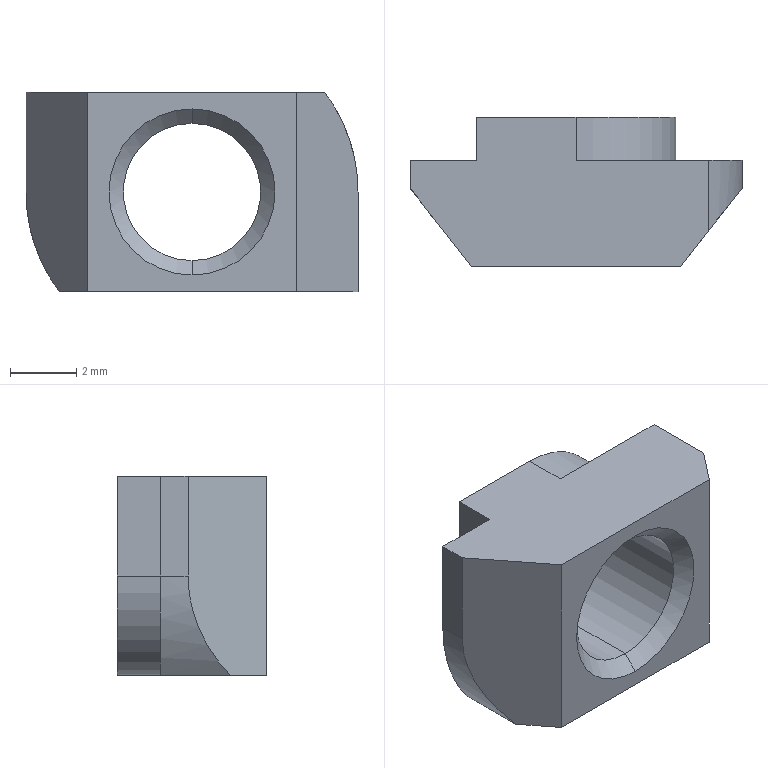Part | SolidWorks | features ICE 2, Extrusion 1, Fillet 1, RevCut 1 | 1 solid | 22 faces | box 10 x 4.5 x 6 mm | volume 142.178 mm3 | plane 12 | cylinder 6 | cone 4 | commonest cylinder face diameters 4.134 x2 6 x2 10 x2
STEP:
#1=CARTESIAN_POINT('',(0.,4.067,5.067));
#2=VERTEX_POINT('',#1);
#3=CARTESIAN_POINT('',(0.,4.067,0.933));
#4=VERTEX_POINT('',#3);
#5=CARTESIAN_POINT('',(0.,4.067,3.));
#6=DIRECTION('',(0.,-1.,0.));
#7=DIRECTION('',(0.,0.,-1.));
#8=AXIS2_PLACEMENT_3D('',#5,#6,#7);
#9=CIRCLE('',#8,2.067);
#10=EDGE_CURVE('',#2,#4,#9,.T.);
#11=ORIENTED_EDGE('',*,*,#10,.T.);
#12=CARTESIAN_POINT('',(0.,4.5,0.5));
#13=VERTEX_POINT('',#12);
#14=CARTESIAN_POINT('',(0.,4.5,0.5));
#15=DIRECTION('',(0.,0.7071,-0.7071));
#16=VECTOR('',#15,1000.);
#17=LINE('',#14,#16);
#18=EDGE_CURVE('',#4,#13,#17,.T.);
#19=ORIENTED_EDGE('',*,*,#18,.T.);
#20=CARTESIAN_POINT('',(0.,4.5,5.5));
#21=VERTEX_POINT('',#20);
#22=CARTESIAN_POINT('',(0.,4.5,3.));
#23=DIRECTION('',(0.,-1.,0.));
#24=DIRECTION('',(0.,0.,-1.));
#25=AXIS2_PLACEMENT_3D('',#22,#23,#24);
#26=CIRCLE('',#25,2.5);
#27=EDGE_CURVE('',#21,#13,#26,.T.);
#28=ORIENTED_EDGE('',*,*,#27,.F.);
#29=CARTESIAN_POINT('',(0.,4.5,5.5));
#30=DIRECTION('',(0.,0.7071,0.7071));
#31=VECTOR('',#30,1000.);
#32=LINE('',#29,#31);
#33=EDGE_CURVE('',#2,#21,#32,.T.);
#34=ORIENTED_EDGE('',*,*,#33,.F.);
#35=EDGE_LOOP('',(#11,#19,#28,#34));
#36=FACE_OUTER_BOUND('',#35,.T.);
#37=CARTESIAN_POINT('',(0.,4.5,3.));
#38=DIRECTION('',(0.,1.,0.));
#39=DIRECTION('',(0.,0.,1.));
#40=AXIS2_PLACEMENT_3D('',#37,#38,#39);
#41=CONICAL_SURFACE('',#40,2.5,0.7854);
#42=ADVANCED_FACE('',(#36),#41,.F.);
#43=ORIENTED_EDGE('',*,*,#10,.F.);
#44=CARTESIAN_POINT('',(0.,0.433,5.067));
#45=VERTEX_POINT('',#44);
#46=CARTESIAN_POINT('',(0.,50.,5.067));
#47=DIRECTION('',(0.,-1.,0.));
#48=VECTOR('',#47,1000.);
#49=LINE('',#46,#48);
#50=EDGE_CURVE('',#2,#45,#49,.T.);
#51=ORIENTED_EDGE('',*,*,#50,.T.);
#52=CARTESIAN_POINT('',(0.,0.433,0.933));
#53=VERTEX_POINT('',#52);
#54=CARTESIAN_POINT('',(0.,0.433,3.));
#55=DIRECTION('',(0.,-1.,0.));
#56=DIRECTION('',(0.,0.,-1.));
#57=AXIS2_PLACEMENT_3D('',#54,#55,#56);
#58=CIRCLE('',#57,2.067);
#59=EDGE_CURVE('',#45,#53,#58,.T.);
#60=ORIENTED_EDGE('',*,*,#59,.T.);
#61=CARTESIAN_POINT('',(0.,50.,0.933));
#62=DIRECTION('',(0.,-1.,0.));
#63=VECTOR('',#62,1000.);
#64=LINE('',#61,#63);
#65=EDGE_CURVE('',#4,#53,#64,.T.);
#66=ORIENTED_EDGE('',*,*,#65,.F.);
#67=EDGE_LOOP('',(#43,#51,#60,#66));
#68=FACE_OUTER_BOUND('',#67,.T.);
#69=CARTESIAN_POINT('',(0.,50.,3.));
#70=DIRECTION('',(0.,-1.,0.));
#71=DIRECTION('',(0.,0.,-1.));
#72=AXIS2_PLACEMENT_3D('',#69,#70,#71);
#73=CYLINDRICAL_SURFACE('',#72,2.067);
#74=ADVANCED_FACE('',(#68),#73,.F.);
#75=ORIENTED_EDGE('',*,*,#59,.F.);
#76=CARTESIAN_POINT('',(0.,0.,5.5));
#77=VERTEX_POINT('',#76);
#78=CARTESIAN_POINT('',(0.,0.433,5.067));
#79=DIRECTION('',(0.,-0.7071,0.7071));
#80=VECTOR('',#79,1000.);
#81=LINE('',#78,#80);
#82=EDGE_CURVE('',#45,#77,#81,.T.);
#83=ORIENTED_EDGE('',*,*,#82,.T.);
#84=CARTESIAN_POINT('',(0.,0.,0.5));
#85=VERTEX_POINT('',#84);
#86=CARTESIAN_POINT('',(0.,0.,3.));
#87=DIRECTION('',(0.,-1.,0.));
#88=DIRECTION('',(0.,0.,-1.));
#89=AXIS2_PLACEMENT_3D('',#86,#87,#88);
#90=CIRCLE('',#89,2.5);
#91=EDGE_CURVE('',#77,#85,#90,.T.);
#92=ORIENTED_EDGE('',*,*,#91,.T.);
#93=CARTESIAN_POINT('',(0.,0.433,0.933));
#94=DIRECTION('',(0.,-0.7071,-0.7071));
#95=VECTOR('',#94,1000.);
#96=LINE('',#93,#95);
#97=EDGE_CURVE('',#53,#85,#96,.T.);
#98=ORIENTED_EDGE('',*,*,#97,.F.);
#99=EDGE_LOOP('',(#75,#83,#92,#98));
#100=FACE_OUTER_BOUND('',#99,.T.);
#101=CARTESIAN_POINT('',(0.,0.433,3.));
#102=DIRECTION('',(0.,-1.,0.));
#103=DIRECTION('',(0.,0.,-1.));
#104=AXIS2_PLACEMENT_3D('',#101,#102,#103);
#105=CONICAL_SURFACE('',#104,2.067,0.7854);
#106=ADVANCED_FACE('',(#100),#105,.F.);
#107=CARTESIAN_POINT('',(-5.,3.2,6.));
#108=VERTEX_POINT('',#107);
#109=CARTESIAN_POINT('',(-5.,3.2,3.));
#110=VERTEX_POINT('',#109);
#111=CARTESIAN_POINT('',(-5.,3.2,6.));
#112=DIRECTION('',(0.,0.,-1.));
#113=VECTOR('',#112,1000.);
#114=LINE('',#111,#113);
#115=EDGE_CURVE('',#108,#110,#114,.T.);
#116=ORIENTED_EDGE('',*,*,#115,.T.);
#117=CARTESIAN_POINT('',(-5.,2.368,3.));
#118=VERTEX_POINT('',#117);
#119=CARTESIAN_POINT('',(-5.,0.,3.));
#120=DIRECTION('',(0.,1.,0.));
#121=VECTOR('',#120,1000.);
#122=LINE('',#119,#121);
#123=EDGE_CURVE('',#118,#110,#122,.T.);
#124=ORIENTED_EDGE('',*,*,#123,.F.);
#125=CARTESIAN_POINT('',(-5.,2.368,6.));
#126=VERTEX_POINT('',#125);
#127=CARTESIAN_POINT('',(-5.,2.368,6.));
#128=DIRECTION('',(0.,0.,-1.));
#129=VECTOR('',#128,1000.);
#130=LINE('',#127,#129);
#131=EDGE_CURVE('',#126,#118,#130,.T.);
#132=ORIENTED_EDGE('',*,*,#131,.F.);
#133=CARTESIAN_POINT('',(-5.,3.2,6.));
#134=DIRECTION('',(0.,-1.,0.));
#135=VECTOR('',#134,1000.);
#136=LINE('',#133,#135);
#137=EDGE_CURVE('',#108,#126,#136,.T.);
#138=ORIENTED_EDGE('',*,*,#137,.F.);
#139=EDGE_LOOP('',(#116,#124,#132,#138));
#140=FACE_OUTER_BOUND('',#139,.T.);
#141=CARTESIAN_POINT('',(-5.,3.2,6.));
#142=DIRECTION('',(1.,0.,0.));
#143=DIRECTION('',(0.,0.,-1.));
#144=AXIS2_PLACEMENT_3D('',#141,#142,#143);
#145=PLANE('',#144);
#146=ADVANCED_FACE('',(#140),#145,.F.);
#147=ORIENTED_EDGE('',*,*,#131,.T.);
#148=CARTESIAN_POINT('',(-4.,1.088,0.));
#149=VERTEX_POINT('',#148);
#150=CARTESIAN_POINT('',(-5.,2.368,3.));
#151=CARTESIAN_POINT('',(-5.,2.368,1.909));
#152=CARTESIAN_POINT('',(-4.655,1.926,0.8731));
#153=CARTESIAN_POINT('',(-4.,1.088,0.));
#154=(BOUNDED_CURVE()B_SPLINE_CURVE(3,(#150,#151,#152,#153),.UNSPECIFIED.,.F.,.F.)B_SPLINE_CURVE_WITH_KNOTS((4,4),(0.,0.6435),.UNSPECIFIED.)CURVE()GEOMETRIC_REPRESENTATION_ITEM()RATIONAL_B_SPLINE_CURVE((1.,0.9658,0.9658,1.))REPRESENTATION_ITEM(''));
#155=EDGE_CURVE('',#118,#149,#154,.T.);
#156=ORIENTED_EDGE('',*,*,#155,.T.);
#157=CARTESIAN_POINT('',(-3.15,0.,0.));
#158=VERTEX_POINT('',#157);
#159=CARTESIAN_POINT('',(-5.,2.368,0.));
#160=DIRECTION('',(0.6157,-0.788,0.));
#161=VECTOR('',#160,1000.);
#162=LINE('',#159,#161);
#163=EDGE_CURVE('',#149,#158,#162,.T.);
#164=ORIENTED_EDGE('',*,*,#163,.T.);
#165=CARTESIAN_POINT('',(-3.15,0.,6.));
#166=VERTEX_POINT('',#165);
#167=CARTESIAN_POINT('',(-3.15,0.,6.));
#168=DIRECTION('',(0.,0.,-1.));
#169=VECTOR('',#168,1000.);
#170=LINE('',#167,#169);
#171=EDGE_CURVE('',#166,#158,#170,.T.);
#172=ORIENTED_EDGE('',*,*,#171,.F.);
#173=CARTESIAN_POINT('',(-5.,2.368,6.));
#174=DIRECTION('',(0.6157,-0.788,0.));
#175=VECTOR('',#174,1000.);
#176=LINE('',#173,#175);
#177=EDGE_CURVE('',#126,#166,#176,.T.);
#178=ORIENTED_EDGE('',*,*,#177,.F.);
#179=EDGE_LOOP('',(#147,#156,#164,#172,#178));
#180=FACE_OUTER_BOUND('',#179,.T.);
#181=CARTESIAN_POINT('',(-5.,2.368,6.));
#182=DIRECTION('',(0.788,0.6157,0.));
#183=DIRECTION('',(-0.6157,0.788,0.));
#184=AXIS2_PLACEMENT_3D('',#181,#182,#183);
#185=PLANE('',#184);
#186=ADVANCED_FACE('',(#180),#185,.F.);
#187=CARTESIAN_POINT('',(0.,0.,3.));
#188=DIRECTION('',(0.,-1.,0.));
#189=DIRECTION('',(0.,0.,-1.));
#190=AXIS2_PLACEMENT_3D('',#187,#188,#189);
#191=CIRCLE('',#190,2.5);
#192=EDGE_CURVE('',#85,#77,#191,.T.);
#193=ORIENTED_EDGE('',*,*,#192,.F.);
#194=ORIENTED_EDGE('',*,*,#91,.F.);
#195=EDGE_LOOP('',(#193,#194));
#196=FACE_BOUND('',#195,.T.);
#197=CARTESIAN_POINT('',(3.15,0.,0.));
#198=VERTEX_POINT('',#197);
#199=CARTESIAN_POINT('',(-3.15,0.,0.));
#200=DIRECTION('',(1.,0.,0.));
#201=VECTOR('',#200,1000.);
#202=LINE('',#199,#201);
#203=EDGE_CURVE('',#158,#198,#202,.T.);
#204=ORIENTED_EDGE('',*,*,#203,.T.);
#205=CARTESIAN_POINT('',(3.15,0.,6.));
#206=VERTEX_POINT('',#205);
#207=CARTESIAN_POINT('',(3.15,0.,6.));
#208=DIRECTION('',(0.,0.,-1.));
#209=VECTOR('',#208,1000.);
#210=LINE('',#207,#209);
#211=EDGE_CURVE('',#206,#198,#210,.T.);
#212=ORIENTED_EDGE('',*,*,#211,.F.);
#213=CARTESIAN_POINT('',(-3.15,0.,6.));
#214=DIRECTION('',(1.,0.,0.));
#215=VECTOR('',#214,1000.);
#216=LINE('',#213,#215);
#217=EDGE_CURVE('',#166,#206,#216,.T.);
#218=ORIENTED_EDGE('',*,*,#217,.F.);
#219=ORIENTED_EDGE('',*,*,#171,.T.);
#220=EDGE_LOOP('',(#204,#212,#218,#219));
#221=FACE_OUTER_BOUND('',#220,.T.);
#222=CARTESIAN_POINT('',(-3.15,0.,6.));
#223=DIRECTION('',(0.,1.,0.));
#224=DIRECTION('',(0.,0.,1.));
#225=AXIS2_PLACEMENT_3D('',#222,#223,#224);
#226=PLANE('',#225);
#227=ADVANCED_FACE('',(#196,#221),#226,.F.);
#228=CARTESIAN_POINT('',(5.,2.368,3.));
#229=VERTEX_POINT('',#228);
#230=CARTESIAN_POINT('',(5.,2.368,0.));
#231=VERTEX_POINT('',#230);
#232=CARTESIAN_POINT('',(5.,2.368,6.));
#233=DIRECTION('',(0.,0.,-1.));
#234=VECTOR('',#233,1000.);
#235=LINE('',#232,#234);
#236=EDGE_CURVE('',#229,#231,#235,.T.);
#237=ORIENTED_EDGE('',*,*,#236,.F.);
#238=CARTESIAN_POINT('',(4.,1.088,6.));
#239=VERTEX_POINT('',#238);
#240=CARTESIAN_POINT('',(5.,2.368,3.));
#241=CARTESIAN_POINT('',(5.,2.368,4.091));
#242=CARTESIAN_POINT('',(4.655,1.926,5.127));
#243=CARTESIAN_POINT('',(4.,1.088,6.));
#244=(BOUNDED_CURVE()B_SPLINE_CURVE(3,(#240,#241,#242,#243),.UNSPECIFIED.,.F.,.F.)B_SPLINE_CURVE_WITH_KNOTS((4,4),(0.,0.6435),.UNSPECIFIED.)CURVE()GEOMETRIC_REPRESENTATION_ITEM()RATIONAL_B_SPLINE_CURVE((1.,0.9658,0.9658,1.))REPRESENTATION_ITEM(''));
#245=EDGE_CURVE('',#229,#239,#244,.T.);
#246=ORIENTED_EDGE('',*,*,#245,.T.);
#247=CARTESIAN_POINT('',(3.15,0.,6.));
#248=DIRECTION('',(0.6157,0.788,0.));
#249=VECTOR('',#248,1000.);
#250=LINE('',#247,#249);
#251=EDGE_CURVE('',#206,#239,#250,.T.);
#252=ORIENTED_EDGE('',*,*,#251,.F.);
#253=ORIENTED_EDGE('',*,*,#211,.T.);
#254=CARTESIAN_POINT('',(3.15,0.,0.));
#255=DIRECTION('',(0.6157,0.788,0.));
#256=VECTOR('',#255,1000.);
#257=LINE('',#254,#256);
#258=EDGE_CURVE('',#198,#231,#257,.T.);
#259=ORIENTED_EDGE('',*,*,#258,.T.);
#260=EDGE_LOOP('',(#237,#246,#252,#253,#259));
#261=FACE_OUTER_BOUND('',#260,.T.);
#262=CARTESIAN_POINT('',(3.15,0.,6.));
#263=DIRECTION('',(-0.788,0.6157,0.));
#264=DIRECTION('',(-0.6157,-0.788,0.));
#265=AXIS2_PLACEMENT_3D('',#262,#263,#264);
#266=PLANE('',#265);
#267=ADVANCED_FACE('',(#261),#266,.F.);
#268=CARTESIAN_POINT('',(5.,3.2,3.));
#269=VERTEX_POINT('',#268);
#270=CARTESIAN_POINT('',(5.,3.2,0.));
#271=VERTEX_POINT('',#270);
#272=CARTESIAN_POINT('',(5.,3.2,6.));
#273=DIRECTION('',(0.,0.,-1.));
#274=VECTOR('',#273,1000.);
#275=LINE('',#272,#274);
#276=EDGE_CURVE('',#269,#271,#275,.T.);
#277=ORIENTED_EDGE('',*,*,#276,.F.);
#278=CARTESIAN_POINT('',(5.,0.,3.));
#279=DIRECTION('',(0.,1.,0.));
#280=VECTOR('',#279,1000.);
#281=LINE('',#278,#280);
#282=EDGE_CURVE('',#229,#269,#281,.T.);
#283=ORIENTED_EDGE('',*,*,#282,.F.);
#284=ORIENTED_EDGE('',*,*,#236,.T.);
#285=CARTESIAN_POINT('',(5.,2.368,0.));
#286=DIRECTION('',(0.,1.,0.));
#287=VECTOR('',#286,1000.);
#288=LINE('',#285,#287);
#289=EDGE_CURVE('',#231,#271,#288,.T.);
#290=ORIENTED_EDGE('',*,*,#289,.T.);
#291=EDGE_LOOP('',(#277,#283,#284,#290));
#292=FACE_OUTER_BOUND('',#291,.T.);
#293=CARTESIAN_POINT('',(5.,2.368,6.));
#294=DIRECTION('',(-1.,0.,0.));
#295=DIRECTION('',(0.,0.,1.));
#296=AXIS2_PLACEMENT_3D('',#293,#294,#295);
#297=PLANE('',#296);
#298=ADVANCED_FACE('',(#292),#297,.F.);
#299=CARTESIAN_POINT('',(4.,3.2,6.));
#300=VERTEX_POINT('',#299);
#301=CARTESIAN_POINT('',(0.,3.2,6.));
#302=VERTEX_POINT('',#301);
#303=CARTESIAN_POINT('',(5.,3.2,6.));
#304=DIRECTION('',(-1.,0.,0.));
#305=VECTOR('',#304,1000.);
#306=LINE('',#303,#305);
#307=EDGE_CURVE('',#300,#302,#306,.T.);
#308=ORIENTED_EDGE('',*,*,#307,.F.);
#309=CARTESIAN_POINT('',(0.,3.2,3.));
#310=DIRECTION('',(0.,1.,0.));
#311=DIRECTION('',(0.,0.,-1.));
#312=AXIS2_PLACEMENT_3D('',#309,#310,#311);
#313=CIRCLE('',#312,5.);
#314=EDGE_CURVE('',#300,#269,#313,.T.);
#315=ORIENTED_EDGE('',*,*,#314,.T.);
#316=ORIENTED_EDGE('',*,*,#276,.T.);
#317=CARTESIAN_POINT('',(3.,3.2,0.));
#318=VERTEX_POINT('',#317);
#319=CARTESIAN_POINT('',(5.,3.2,0.));
#320=DIRECTION('',(-1.,0.,0.));
#321=VECTOR('',#320,1000.);
#322=LINE('',#319,#321);
#323=EDGE_CURVE('',#271,#318,#322,.T.);
#324=ORIENTED_EDGE('',*,*,#323,.T.);
#325=CARTESIAN_POINT('',(3.,3.2,3.));
#326=VERTEX_POINT('',#325);
#327=CARTESIAN_POINT('',(3.,3.2,6.));
#328=DIRECTION('',(0.,0.,-1.));
#329=VECTOR('',#328,1000.);
#330=LINE('',#327,#329);
#331=EDGE_CURVE('',#326,#318,#330,.T.);
#332=ORIENTED_EDGE('',*,*,#331,.F.);
#333=CARTESIAN_POINT('',(0.,3.2,3.));
#334=DIRECTION('',(0.,-1.,0.));
#335=DIRECTION('',(0.,0.,-1.));
#336=AXIS2_PLACEMENT_3D('',#333,#334,#335);
#337=CIRCLE('',#336,3.);
#338=EDGE_CURVE('',#326,#302,#337,.T.);
#339=ORIENTED_EDGE('',*,*,#338,.T.);
#340=EDGE_LOOP('',(#308,#315,#316,#324,#332,#339));
#341=FACE_OUTER_BOUND('',#340,.T.);
#342=CARTESIAN_POINT('',(5.,3.2,6.));
#343=DIRECTION('',(0.,-1.,0.));
#344=DIRECTION('',(0.,0.,-1.));
#345=AXIS2_PLACEMENT_3D('',#342,#343,#344);
#346=PLANE('',#345);
#347=ADVANCED_FACE('',(#341),#346,.F.);
#348=CARTESIAN_POINT('',(3.,4.5,3.));
#349=VERTEX_POINT('',#348);
#350=CARTESIAN_POINT('',(3.,4.5,0.));
#351=VERTEX_POINT('',#350);
#352=CARTESIAN_POINT('',(3.,4.5,6.));
#353=DIRECTION('',(0.,0.,-1.));
#354=VECTOR('',#353,1000.);
#355=LINE('',#352,#354);
#356=EDGE_CURVE('',#349,#351,#355,.T.);
#357=ORIENTED_EDGE('',*,*,#356,.F.);
#358=CARTESIAN_POINT('',(3.,3.2,3.));
#359=DIRECTION('',(0.,-1.,0.));
#360=VECTOR('',#359,1000.);
#361=LINE('',#358,#360);
#362=EDGE_CURVE('',#349,#326,#361,.T.);
#363=ORIENTED_EDGE('',*,*,#362,.T.);
#364=ORIENTED_EDGE('',*,*,#331,.T.);
#365=CARTESIAN_POINT('',(3.,3.2,0.));
#366=DIRECTION('',(0.,1.,0.));
#367=VECTOR('',#366,1000.);
#368=LINE('',#365,#367);
#369=EDGE_CURVE('',#318,#351,#368,.T.);
#370=ORIENTED_EDGE('',*,*,#369,.T.);
#371=EDGE_LOOP('',(#357,#363,#364,#370));
#372=FACE_OUTER_BOUND('',#371,.T.);
#373=CARTESIAN_POINT('',(3.,3.2,6.));
#374=DIRECTION('',(-1.,0.,0.));
#375=DIRECTION('',(0.,0.,1.));
#376=AXIS2_PLACEMENT_3D('',#373,#374,#375);
#377=PLANE('',#376);
#378=ADVANCED_FACE('',(#372),#377,.F.);
#379=ORIENTED_EDGE('',*,*,#27,.T.);
#380=CARTESIAN_POINT('',(0.,4.5,3.));
#381=DIRECTION('',(0.,-1.,0.));
#382=DIRECTION('',(0.,0.,-1.));
#383=AXIS2_PLACEMENT_3D('',#380,#381,#382);
#384=CIRCLE('',#383,2.5);
#385=EDGE_CURVE('',#13,#21,#384,.T.);
#386=ORIENTED_EDGE('',*,*,#385,.T.);
#387=EDGE_LOOP('',(#379,#386));
#388=FACE_BOUND('',#387,.T.);
#389=CARTESIAN_POINT('',(0.,4.5,6.));
#390=VERTEX_POINT('',#389);
#391=CARTESIAN_POINT('',(-3.,4.5,6.));
#392=VERTEX_POINT('',#391);
#393=CARTESIAN_POINT('',(3.,4.5,6.));
#394=DIRECTION('',(-1.,0.,0.));
#395=VECTOR('',#394,1000.);
#396=LINE('',#393,#395);
#397=EDGE_CURVE('',#390,#392,#396,.T.);
#398=ORIENTED_EDGE('',*,*,#397,.F.);
#399=CARTESIAN_POINT('',(0.,4.5,3.));
#400=DIRECTION('',(0.,1.,0.));
#401=DIRECTION('',(0.,0.,-1.));
#402=AXIS2_PLACEMENT_3D('',#399,#400,#401);
#403=CIRCLE('',#402,3.);
#404=EDGE_CURVE('',#390,#349,#403,.T.);
#405=ORIENTED_EDGE('',*,*,#404,.T.);
#406=ORIENTED_EDGE('',*,*,#356,.T.);
#407=CARTESIAN_POINT('',(0.,4.5,0.));
#408=VERTEX_POINT('',#407);
#409=CARTESIAN_POINT('',(3.,4.5,0.));
#410=DIRECTION('',(-1.,0.,0.));
#411=VECTOR('',#410,1000.);
#412=LINE('',#409,#411);
#413=EDGE_CURVE('',#351,#408,#412,.T.);
#414=ORIENTED_EDGE('',*,*,#413,.T.);
#415=CARTESIAN_POINT('',(-3.,4.5,3.));
#416=VERTEX_POINT('',#415);
#417=CARTESIAN_POINT('',(0.,4.5,3.));
#418=DIRECTION('',(0.,1.,0.));
#419=DIRECTION('',(0.,0.,-1.));
#420=AXIS2_PLACEMENT_3D('',#417,#418,#419);
#421=CIRCLE('',#420,3.);
#422=EDGE_CURVE('',#408,#416,#421,.T.);
#423=ORIENTED_EDGE('',*,*,#422,.T.);
#424=CARTESIAN_POINT('',(-3.,4.5,6.));
#425=DIRECTION('',(0.,0.,-1.));
#426=VECTOR('',#425,1000.);
#427=LINE('',#424,#426);
#428=EDGE_CURVE('',#392,#416,#427,.T.);
#429=ORIENTED_EDGE('',*,*,#428,.F.);
#430=EDGE_LOOP('',(#398,#405,#406,#414,#423,#429));
#431=FACE_OUTER_BOUND('',#430,.T.);
#432=CARTESIAN_POINT('',(3.,4.5,6.));
#433=DIRECTION('',(0.,-1.,0.));
#434=DIRECTION('',(0.,0.,-1.));
#435=AXIS2_PLACEMENT_3D('',#432,#433,#434);
#436=PLANE('',#435);
#437=ADVANCED_FACE('',(#388,#431),#436,.F.);
#438=ORIENTED_EDGE('',*,*,#428,.T.);
#439=CARTESIAN_POINT('',(-3.,3.2,3.));
#440=VERTEX_POINT('',#439);
#441=CARTESIAN_POINT('',(-3.,4.5,3.));
#442=DIRECTION('',(0.,-1.,0.));
#443=VECTOR('',#442,1000.);
#444=LINE('',#441,#443);
#445=EDGE_CURVE('',#416,#440,#444,.T.);
#446=ORIENTED_EDGE('',*,*,#445,.T.);
#447=CARTESIAN_POINT('',(-3.,3.2,6.));
#448=VERTEX_POINT('',#447);
#449=CARTESIAN_POINT('',(-3.,3.2,6.));
#450=DIRECTION('',(0.,0.,-1.));
#451=VECTOR('',#450,1000.);
#452=LINE('',#449,#451);
#453=EDGE_CURVE('',#448,#440,#452,.T.);
#454=ORIENTED_EDGE('',*,*,#453,.F.);
#455=CARTESIAN_POINT('',(-3.,4.5,6.));
#456=DIRECTION('',(0.,-1.,0.));
#457=VECTOR('',#456,1000.);
#458=LINE('',#455,#457);
#459=EDGE_CURVE('',#392,#448,#458,.T.);
#460=ORIENTED_EDGE('',*,*,#459,.F.);
#461=EDGE_LOOP('',(#438,#446,#454,#460));
#462=FACE_OUTER_BOUND('',#461,.T.);
#463=CARTESIAN_POINT('',(-3.,4.5,6.));
#464=DIRECTION('',(1.,0.,0.));
#465=DIRECTION('',(0.,0.,-1.));
#466=AXIS2_PLACEMENT_3D('',#463,#464,#465);
#467=PLANE('',#466);
#468=ADVANCED_FACE('',(#462),#467,.F.);
#469=CARTESIAN_POINT('',(0.,3.2,0.));
#470=VERTEX_POINT('',#469);
#471=CARTESIAN_POINT('',(-4.,3.2,0.));
#472=VERTEX_POINT('',#471);
#473=CARTESIAN_POINT('',(-3.,3.2,0.));
#474=DIRECTION('',(-1.,0.,0.));
#475=VECTOR('',#474,1000.);
#476=LINE('',#473,#475);
#477=EDGE_CURVE('',#470,#472,#476,.T.);
#478=ORIENTED_EDGE('',*,*,#477,.T.);
#479=CARTESIAN_POINT('',(0.,3.2,3.));
#480=DIRECTION('',(0.,1.,0.));
#481=DIRECTION('',(0.,0.,-1.));
#482=AXIS2_PLACEMENT_3D('',#479,#480,#481);
#483=CIRCLE('',#482,5.);
#484=EDGE_CURVE('',#472,#110,#483,.T.);
#485=ORIENTED_EDGE('',*,*,#484,.T.);
#486=ORIENTED_EDGE('',*,*,#115,.F.);
#487=CARTESIAN_POINT('',(-3.,3.2,6.));
#488=DIRECTION('',(-1.,0.,0.));
#489=VECTOR('',#488,1000.);
#490=LINE('',#487,#489);
#491=EDGE_CURVE('',#448,#108,#490,.T.);
#492=ORIENTED_EDGE('',*,*,#491,.F.);
#493=ORIENTED_EDGE('',*,*,#453,.T.);
#494=CARTESIAN_POINT('',(0.,3.2,3.));
#495=DIRECTION('',(0.,-1.,0.));
#496=DIRECTION('',(0.,0.,-1.));
#497=AXIS2_PLACEMENT_3D('',#494,#495,#496);
#498=CIRCLE('',#497,3.);
#499=EDGE_CURVE('',#440,#470,#498,.T.);
#500=ORIENTED_EDGE('',*,*,#499,.T.);
#501=EDGE_LOOP('',(#478,#485,#486,#492,#493,#500));
#502=FACE_OUTER_BOUND('',#501,.T.);
#503=CARTESIAN_POINT('',(-3.,3.2,6.));
#504=DIRECTION('',(0.,-1.,0.));
#505=DIRECTION('',(0.,0.,-1.));
#506=AXIS2_PLACEMENT_3D('',#503,#504,#505);
#507=PLANE('',#506);
#508=ADVANCED_FACE('',(#502),#507,.F.);
#509=ORIENTED_EDGE('',*,*,#307,.T.);
#510=CARTESIAN_POINT('',(0.,4.5,6.));
#511=DIRECTION('',(0.,1.,0.));
#512=VECTOR('',#511,1000.);
#513=LINE('',#510,#512);
#514=EDGE_CURVE('',#302,#390,#513,.T.);
#515=ORIENTED_EDGE('',*,*,#514,.T.);
#516=ORIENTED_EDGE('',*,*,#397,.T.);
#517=ORIENTED_EDGE('',*,*,#459,.T.);
#518=ORIENTED_EDGE('',*,*,#491,.T.);
#519=ORIENTED_EDGE('',*,*,#137,.T.);
#520=ORIENTED_EDGE('',*,*,#177,.T.);
#521=ORIENTED_EDGE('',*,*,#217,.T.);
#522=ORIENTED_EDGE('',*,*,#251,.T.);
#523=CARTESIAN_POINT('',(4.,0.,6.));
#524=DIRECTION('',(0.,-1.,0.));
#525=VECTOR('',#524,1000.);
#526=LINE('',#523,#525);
#527=EDGE_CURVE('',#300,#239,#526,.T.);
#528=ORIENTED_EDGE('',*,*,#527,.F.);
#529=EDGE_LOOP('',(#509,#515,#516,#517,#518,#519,#520,#521,#522,#528));
#530=FACE_OUTER_BOUND('',#529,.T.);
#531=CARTESIAN_POINT('',(0.,0.,6.));
#532=DIRECTION('',(0.,0.,1.));
#533=DIRECTION('',(1.,0.,0.));
#534=AXIS2_PLACEMENT_3D('',#531,#532,#533);
#535=PLANE('',#534);
#536=ADVANCED_FACE('',(#530),#535,.T.);
#537=ORIENTED_EDGE('',*,*,#477,.F.);
#538=CARTESIAN_POINT('',(0.,0.,0.));
#539=DIRECTION('',(0.,1.,0.));
#540=VECTOR('',#539,1000.);
#541=LINE('',#538,#540);
#542=EDGE_CURVE('',#470,#408,#541,.T.);
#543=ORIENTED_EDGE('',*,*,#542,.T.);
#544=ORIENTED_EDGE('',*,*,#413,.F.);
#545=ORIENTED_EDGE('',*,*,#369,.F.);
#546=ORIENTED_EDGE('',*,*,#323,.F.);
#547=ORIENTED_EDGE('',*,*,#289,.F.);
#548=ORIENTED_EDGE('',*,*,#258,.F.);
#549=ORIENTED_EDGE('',*,*,#203,.F.);
#550=ORIENTED_EDGE('',*,*,#163,.F.);
#551=CARTESIAN_POINT('',(-4.,0.,0.));
#552=DIRECTION('',(0.,1.,0.));
#553=VECTOR('',#552,1000.);
#554=LINE('',#551,#553);
#555=EDGE_CURVE('',#149,#472,#554,.T.);
#556=ORIENTED_EDGE('',*,*,#555,.T.);
#557=EDGE_LOOP('',(#537,#543,#544,#545,#546,#547,#548,#549,#550,#556));
#558=FACE_OUTER_BOUND('',#557,.T.);
#559=CARTESIAN_POINT('',(0.,0.,0.));
#560=DIRECTION('',(0.,0.,1.));
#561=DIRECTION('',(1.,0.,0.));
#562=AXIS2_PLACEMENT_3D('',#559,#560,#561);
#563=PLANE('',#562);
#564=ADVANCED_FACE('',(#558),#563,.F.);
#565=ORIENTED_EDGE('',*,*,#82,.F.);
#566=CARTESIAN_POINT('',(0.,0.433,3.));
#567=DIRECTION('',(0.,-1.,0.));
#568=DIRECTION('',(0.,0.,-1.));
#569=AXIS2_PLACEMENT_3D('',#566,#567,#568);
#570=CIRCLE('',#569,2.067);
#571=EDGE_CURVE('',#53,#45,#570,.T.);
#572=ORIENTED_EDGE('',*,*,#571,.F.);
#573=ORIENTED_EDGE('',*,*,#97,.T.);
#574=ORIENTED_EDGE('',*,*,#192,.T.);
#575=EDGE_LOOP('',(#565,#572,#573,#574));
#576=FACE_OUTER_BOUND('',#575,.T.);
#577=CARTESIAN_POINT('',(0.,0.433,3.));
#578=DIRECTION('',(0.,-1.,0.));
#579=DIRECTION('',(0.,0.,-1.));
#580=AXIS2_PLACEMENT_3D('',#577,#578,#579);
#581=CONICAL_SURFACE('',#580,2.067,0.7854);
#582=ADVANCED_FACE('',(#576),#581,.F.);
#583=ORIENTED_EDGE('',*,*,#50,.F.);
#584=CARTESIAN_POINT('',(0.,4.067,3.));
#585=DIRECTION('',(0.,-1.,0.));
#586=DIRECTION('',(0.,0.,-1.));
#587=AXIS2_PLACEMENT_3D('',#584,#585,#586);
#588=CIRCLE('',#587,2.067);
#589=EDGE_CURVE('',#4,#2,#588,.T.);
#590=ORIENTED_EDGE('',*,*,#589,.F.);
#591=ORIENTED_EDGE('',*,*,#65,.T.);
#592=ORIENTED_EDGE('',*,*,#571,.T.);
#593=EDGE_LOOP('',(#583,#590,#591,#592));
#594=FACE_OUTER_BOUND('',#593,.T.);
#595=CARTESIAN_POINT('',(0.,50.,3.));
#596=DIRECTION('',(0.,-1.,0.));
#597=DIRECTION('',(0.,0.,-1.));
#598=AXIS2_PLACEMENT_3D('',#595,#596,#597);
#599=CYLINDRICAL_SURFACE('',#598,2.067);
#600=ADVANCED_FACE('',(#594),#599,.F.);
#601=ORIENTED_EDGE('',*,*,#18,.F.);
#602=ORIENTED_EDGE('',*,*,#589,.T.);
#603=ORIENTED_EDGE('',*,*,#33,.T.);
#604=ORIENTED_EDGE('',*,*,#385,.F.);
#605=EDGE_LOOP('',(#601,#602,#603,#604));
#606=FACE_OUTER_BOUND('',#605,.T.);
#607=CARTESIAN_POINT('',(0.,4.5,3.));
#608=DIRECTION('',(0.,1.,0.));
#609=DIRECTION('',(0.,0.,1.));
#610=AXIS2_PLACEMENT_3D('',#607,#608,#609);
#611=CONICAL_SURFACE('',#610,2.5,0.7854);
#612=ADVANCED_FACE('',(#606),#611,.F.);
#613=ORIENTED_EDGE('',*,*,#282,.T.);
#614=ORIENTED_EDGE('',*,*,#314,.F.);
#615=ORIENTED_EDGE('',*,*,#527,.T.);
#616=ORIENTED_EDGE('',*,*,#245,.F.);
#617=EDGE_LOOP('',(#613,#614,#615,#616));
#618=FACE_OUTER_BOUND('',#617,.T.);
#619=CARTESIAN_POINT('',(0.,0.,3.));
#620=DIRECTION('',(0.,1.,0.));
#621=DIRECTION('',(0.,0.,1.));
#622=AXIS2_PLACEMENT_3D('',#619,#620,#621);
#623=CYLINDRICAL_SURFACE('',#622,5.);
#624=ADVANCED_FACE('',(#618),#623,.T.);
#625=ORIENTED_EDGE('',*,*,#123,.T.);
#626=ORIENTED_EDGE('',*,*,#484,.F.);
#627=ORIENTED_EDGE('',*,*,#555,.F.);
#628=ORIENTED_EDGE('',*,*,#155,.F.);
#629=EDGE_LOOP('',(#625,#626,#627,#628));
#630=FACE_OUTER_BOUND('',#629,.T.);
#631=CARTESIAN_POINT('',(0.,0.,3.));
#632=DIRECTION('',(0.,1.,0.));
#633=DIRECTION('',(0.,0.,1.));
#634=AXIS2_PLACEMENT_3D('',#631,#632,#633);
#635=CYLINDRICAL_SURFACE('',#634,5.);
#636=ADVANCED_FACE('',(#630),#635,.T.);
#637=ORIENTED_EDGE('',*,*,#338,.F.);
#638=ORIENTED_EDGE('',*,*,#362,.F.);
#639=ORIENTED_EDGE('',*,*,#404,.F.);
#640=ORIENTED_EDGE('',*,*,#514,.F.);
#641=EDGE_LOOP('',(#637,#638,#639,#640));
#642=FACE_OUTER_BOUND('',#641,.T.);
#643=CARTESIAN_POINT('',(0.,0.,3.));
#644=DIRECTION('',(0.,-1.,0.));
#645=DIRECTION('',(0.,0.,-1.));
#646=AXIS2_PLACEMENT_3D('',#643,#644,#645);
#647=CYLINDRICAL_SURFACE('',#646,3.);
#648=ADVANCED_FACE('',(#642),#647,.T.);
#649=ORIENTED_EDGE('',*,*,#422,.F.);
#650=ORIENTED_EDGE('',*,*,#542,.F.);
#651=ORIENTED_EDGE('',*,*,#499,.F.);
#652=ORIENTED_EDGE('',*,*,#445,.F.);
#653=EDGE_LOOP('',(#649,#650,#651,#652));
#654=FACE_OUTER_BOUND('',#653,.T.);
#655=CARTESIAN_POINT('',(0.,4.5,3.));
#656=DIRECTION('',(0.,-1.,0.));
#657=DIRECTION('',(0.,0.,-1.));
#658=AXIS2_PLACEMENT_3D('',#655,#656,#657);
#659=CYLINDRICAL_SURFACE('',#658,3.);
#660=ADVANCED_FACE('',(#654),#659,.T.);
#661=CLOSED_SHELL('',(#42,#74,#106,#146,#186,#227,#267,#298,#347,#378,#437,#468,#508,#536,#564,#582,#600,#612,#624,#636,#648,#660));
#662=MANIFOLD_SOLID_BREP('',#661);
#663=CARTESIAN_POINT('',(0.,0.,0.));
#664=DIRECTION('',(0.,0.,1.));
#665=DIRECTION('',(1.,0.,0.));
#666=AXIS2_PLACEMENT_3D('',#663,#664,#665);
#667=(LENGTH_UNIT()NAMED_UNIT(*)SI_UNIT(.MILLI.,.METRE.));
#668=UNCERTAINTY_MEASURE_WITH_UNIT(LENGTH_MEASURE(0.00001),#667,'','');
#669=(NAMED_UNIT(*)PLANE_ANGLE_UNIT()SI_UNIT($,.RADIAN.));
#670=(NAMED_UNIT(*)SI_UNIT($,.STERADIAN.)SOLID_ANGLE_UNIT());
#671=(GEOMETRIC_REPRESENTATION_CONTEXT(3)GLOBAL_UNCERTAINTY_ASSIGNED_CONTEXT((#668))GLOBAL_UNIT_ASSIGNED_CONTEXT((#667,#669,#670))REPRESENTATION_CONTEXT('',''));
#672=ADVANCED_BREP_SHAPE_REPRESENTATION('',(#662,#666),#671);